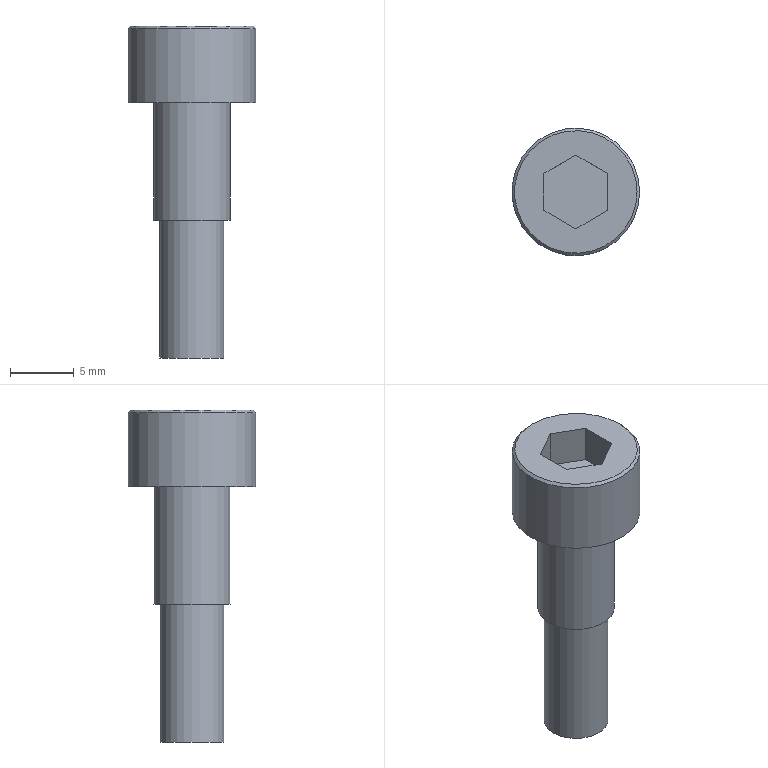Part | STEP file | M3-10_id562_x_t | 1 solid | 15 faces | box 10 x 10 x 26 mm | volume 877.848 mm3 | plane 11 | cylinder 3 | cone 1 | commonest cylinder face diameters 5 x1 6 x1 10 x1
STEP:
#1=CARTESIAN_POINT('',(-317.5,-147.5,-54.182));
#2=VERTEX_POINT('',#1);
#3=CARTESIAN_POINT('',(-315.,-147.5,-54.182));
#4=DIRECTION('',(0.,0.,-1.));
#5=DIRECTION('',(-1.,0.,0.));
#6=AXIS2_PLACEMENT_3D('',#3,#4,#5);
#7=CIRCLE('',#6,2.5);
#8=EDGE_CURVE('',#2,#2,#7,.T.);
#9=ORIENTED_EDGE('',*,*,#8,.F.);
#10=EDGE_LOOP('',(#9));
#11=FACE_BOUND('',#10,.T.);
#12=CARTESIAN_POINT('',(-312.,-147.5,-54.182));
#13=VERTEX_POINT('',#12);
#14=CARTESIAN_POINT('',(-315.,-147.5,-54.182));
#15=DIRECTION('',(0.,0.,1.));
#16=DIRECTION('',(1.,0.,0.));
#17=AXIS2_PLACEMENT_3D('',#14,#15,#16);
#18=CIRCLE('',#17,3.);
#19=EDGE_CURVE('',#13,#13,#18,.T.);
#20=ORIENTED_EDGE('',*,*,#19,.F.);
#21=EDGE_LOOP('',(#20));
#22=FACE_BOUND('',#21,.T.);
#23=CARTESIAN_POINT('',(-315.,-147.5,-54.182));
#24=DIRECTION('',(0.,0.,-1.));
#25=DIRECTION('',(-1.,0.,0.));
#26=AXIS2_PLACEMENT_3D('',#23,#24,#25);
#27=PLANE('',#26);
#28=ADVANCED_FACE('',(#11,#22),#27,.T.);
#29=CARTESIAN_POINT('',(-318.,-147.5,-44.982));
#30=VERTEX_POINT('',#29);
#31=CARTESIAN_POINT('',(-315.,-147.5,-44.982));
#32=DIRECTION('',(0.,0.,1.));
#33=DIRECTION('',(-1.,0.,0.));
#34=AXIS2_PLACEMENT_3D('',#31,#32,#33);
#35=CIRCLE('',#34,3.);
#36=EDGE_CURVE('',#30,#30,#35,.T.);
#37=ORIENTED_EDGE('',*,*,#36,.F.);
#38=EDGE_LOOP('',(#37));
#39=FACE_BOUND('',#38,.T.);
#40=ORIENTED_EDGE('',*,*,#19,.T.);
#41=EDGE_LOOP('',(#40));
#42=FACE_BOUND('',#41,.T.);
#43=CARTESIAN_POINT('',(-315.,-147.5,-54.182));
#44=DIRECTION('',(0.,0.,1.));
#45=DIRECTION('',(1.,0.,0.));
#46=AXIS2_PLACEMENT_3D('',#43,#44,#45);
#47=CYLINDRICAL_SURFACE('',#46,3.);
#48=ADVANCED_FACE('',(#39,#42),#47,.T.);
#49=CARTESIAN_POINT('',(-312.5,-147.5,-64.982));
#50=VERTEX_POINT('',#49);
#51=CARTESIAN_POINT('',(-315.,-147.5,-64.982));
#52=DIRECTION('',(0.,0.,1.));
#53=DIRECTION('',(1.,0.,0.));
#54=AXIS2_PLACEMENT_3D('',#51,#52,#53);
#55=CIRCLE('',#54,2.5);
#56=EDGE_CURVE('',#50,#50,#55,.T.);
#57=ORIENTED_EDGE('',*,*,#56,.F.);
#58=EDGE_LOOP('',(#57));
#59=FACE_OUTER_BOUND('',#58,.T.);
#60=CARTESIAN_POINT('',(-315.,-147.5,-64.982));
#61=DIRECTION('',(0.,0.,-1.));
#62=DIRECTION('',(-1.,0.,0.));
#63=AXIS2_PLACEMENT_3D('',#60,#61,#62);
#64=PLANE('',#63);
#65=ADVANCED_FACE('',(#59),#64,.T.);
#66=ORIENTED_EDGE('',*,*,#56,.T.);
#67=EDGE_LOOP('',(#66));
#68=FACE_BOUND('',#67,.T.);
#69=ORIENTED_EDGE('',*,*,#8,.T.);
#70=EDGE_LOOP('',(#69));
#71=FACE_BOUND('',#70,.T.);
#72=CARTESIAN_POINT('',(-315.,-147.5,-54.182));
#73=DIRECTION('',(0.,0.,-1.));
#74=DIRECTION('',(1.,0.,0.));
#75=AXIS2_PLACEMENT_3D('',#72,#73,#74);
#76=CYLINDRICAL_SURFACE('',#75,2.5);
#77=ADVANCED_FACE('',(#68,#71),#76,.T.);
#78=CARTESIAN_POINT('',(-317.5,-146.057,-38.982));
#79=VERTEX_POINT('',#78);
#80=CARTESIAN_POINT('',(-317.5,-148.943,-38.982));
#81=VERTEX_POINT('',#80);
#82=CARTESIAN_POINT('',(-317.5,-146.057,-38.982));
#83=DIRECTION('',(0.,-1.,0.));
#84=VECTOR('',#83,1.);
#85=LINE('',#82,#84);
#86=EDGE_CURVE('',#79,#81,#85,.T.);
#87=ORIENTED_EDGE('',*,*,#86,.F.);
#88=CARTESIAN_POINT('',(-315.,-144.613,-38.982));
#89=VERTEX_POINT('',#88);
#90=CARTESIAN_POINT('',(-315.,-144.613,-38.982));
#91=DIRECTION('',(-0.866,-0.5,0.));
#92=VECTOR('',#91,1.);
#93=LINE('',#90,#92);
#94=EDGE_CURVE('',#89,#79,#93,.T.);
#95=ORIENTED_EDGE('',*,*,#94,.F.);
#96=CARTESIAN_POINT('',(-312.5,-146.057,-38.982));
#97=VERTEX_POINT('',#96);
#98=CARTESIAN_POINT('',(-312.5,-146.057,-38.982));
#99=DIRECTION('',(-0.866,0.5,0.));
#100=VECTOR('',#99,1.);
#101=LINE('',#98,#100);
#102=EDGE_CURVE('',#97,#89,#101,.T.);
#103=ORIENTED_EDGE('',*,*,#102,.F.);
#104=CARTESIAN_POINT('',(-312.5,-148.943,-38.982));
#105=VERTEX_POINT('',#104);
#106=CARTESIAN_POINT('',(-312.5,-148.943,-38.982));
#107=DIRECTION('',(0.,1.,0.));
#108=VECTOR('',#107,1.);
#109=LINE('',#106,#108);
#110=EDGE_CURVE('',#105,#97,#109,.T.);
#111=ORIENTED_EDGE('',*,*,#110,.F.);
#112=CARTESIAN_POINT('',(-315.,-150.387,-38.982));
#113=VERTEX_POINT('',#112);
#114=CARTESIAN_POINT('',(-315.,-150.387,-38.982));
#115=DIRECTION('',(0.866,0.5,0.));
#116=VECTOR('',#115,1.);
#117=LINE('',#114,#116);
#118=EDGE_CURVE('',#113,#105,#117,.T.);
#119=ORIENTED_EDGE('',*,*,#118,.F.);
#120=CARTESIAN_POINT('',(-317.5,-148.943,-38.982));
#121=DIRECTION('',(0.866,-0.5,0.));
#122=VECTOR('',#121,1.);
#123=LINE('',#120,#122);
#124=EDGE_CURVE('',#81,#113,#123,.T.);
#125=ORIENTED_EDGE('',*,*,#124,.F.);
#126=EDGE_LOOP('',(#87,#95,#103,#111,#119,#125));
#127=FACE_BOUND('',#126,.T.);
#128=CARTESIAN_POINT('',(-310.2,-147.5,-38.982));
#129=VERTEX_POINT('',#128);
#130=CARTESIAN_POINT('',(-315.,-147.5,-38.982));
#131=DIRECTION('',(0.,0.,1.));
#132=DIRECTION('',(1.,0.,0.));
#133=AXIS2_PLACEMENT_3D('',#130,#131,#132);
#134=CIRCLE('',#133,4.8);
#135=EDGE_CURVE('',#129,#129,#134,.T.);
#136=ORIENTED_EDGE('',*,*,#135,.T.);
#137=EDGE_LOOP('',(#136));
#138=FACE_BOUND('',#137,.T.);
#139=CARTESIAN_POINT('',(-315.,-147.5,-38.982));
#140=DIRECTION('',(0.,0.,1.));
#141=DIRECTION('',(1.,0.,0.));
#142=AXIS2_PLACEMENT_3D('',#139,#140,#141);
#143=PLANE('',#142);
#144=ADVANCED_FACE('',(#127,#138),#143,.T.);
#145=ORIENTED_EDGE('',*,*,#36,.T.);
#146=EDGE_LOOP('',(#145));
#147=FACE_BOUND('',#146,.T.);
#148=CARTESIAN_POINT('',(-310.,-147.5,-44.982));
#149=VERTEX_POINT('',#148);
#150=CARTESIAN_POINT('',(-315.,-147.5,-44.982));
#151=DIRECTION('',(0.,0.,1.));
#152=DIRECTION('',(1.,0.,0.));
#153=AXIS2_PLACEMENT_3D('',#150,#151,#152);
#154=CIRCLE('',#153,5.);
#155=EDGE_CURVE('',#149,#149,#154,.T.);
#156=ORIENTED_EDGE('',*,*,#155,.F.);
#157=EDGE_LOOP('',(#156));
#158=FACE_BOUND('',#157,.T.);
#159=CARTESIAN_POINT('',(-315.,-147.5,-44.982));
#160=DIRECTION('',(0.,0.,-1.));
#161=DIRECTION('',(-1.,0.,0.));
#162=AXIS2_PLACEMENT_3D('',#159,#160,#161);
#163=PLANE('',#162);
#164=ADVANCED_FACE('',(#147,#158),#163,.T.);
#165=CARTESIAN_POINT('',(-310.,-147.5,-39.182));
#166=VERTEX_POINT('',#165);
#167=CARTESIAN_POINT('',(-315.,-147.5,-39.182));
#168=DIRECTION('',(0.,0.,-1.));
#169=DIRECTION('',(1.,0.,0.));
#170=AXIS2_PLACEMENT_3D('',#167,#168,#169);
#171=CIRCLE('',#170,5.);
#172=EDGE_CURVE('',#166,#166,#171,.T.);
#173=ORIENTED_EDGE('',*,*,#172,.T.);
#174=EDGE_LOOP('',(#173));
#175=FACE_BOUND('',#174,.T.);
#176=ORIENTED_EDGE('',*,*,#155,.T.);
#177=EDGE_LOOP('',(#176));
#178=FACE_BOUND('',#177,.T.);
#179=CARTESIAN_POINT('',(-315.,-147.5,-44.982));
#180=DIRECTION('',(0.,0.,1.));
#181=DIRECTION('',(1.,0.,0.));
#182=AXIS2_PLACEMENT_3D('',#179,#180,#181);
#183=CYLINDRICAL_SURFACE('',#182,5.);
#184=ADVANCED_FACE('',(#175,#178),#183,.T.);
#185=ORIENTED_EDGE('',*,*,#135,.F.);
#186=EDGE_LOOP('',(#185));
#187=FACE_BOUND('',#186,.T.);
#188=ORIENTED_EDGE('',*,*,#172,.F.);
#189=EDGE_LOOP('',(#188));
#190=FACE_BOUND('',#189,.T.);
#191=CARTESIAN_POINT('',(-315.,-147.5,-39.182));
#192=DIRECTION('',(0.,0.,-1.));
#193=DIRECTION('',(-1.,0.,0.));
#194=AXIS2_PLACEMENT_3D('',#191,#192,#193);
#195=CONICAL_SURFACE('',#194,5.,45.);
#196=ADVANCED_FACE('',(#187,#190),#195,.T.);
#197=ORIENTED_EDGE('',*,*,#86,.T.);
#198=CARTESIAN_POINT('',(-317.5,-148.943,-41.982));
#199=VERTEX_POINT('',#198);
#200=CARTESIAN_POINT('',(-317.5,-148.943,-41.982));
#201=DIRECTION('',(0.,0.,-1.));
#202=VECTOR('',#201,1.);
#203=LINE('',#200,#202);
#204=EDGE_CURVE('',#81,#199,#203,.T.);
#205=ORIENTED_EDGE('',*,*,#204,.T.);
#206=CARTESIAN_POINT('',(-317.5,-146.057,-41.982));
#207=VERTEX_POINT('',#206);
#208=CARTESIAN_POINT('',(-317.5,-146.057,-41.982));
#209=DIRECTION('',(0.,1.,0.));
#210=VECTOR('',#209,1.);
#211=LINE('',#208,#210);
#212=EDGE_CURVE('',#199,#207,#211,.T.);
#213=ORIENTED_EDGE('',*,*,#212,.T.);
#214=CARTESIAN_POINT('',(-317.5,-146.057,-41.982));
#215=DIRECTION('',(0.,0.,-1.));
#216=VECTOR('',#215,1.);
#217=LINE('',#214,#216);
#218=EDGE_CURVE('',#79,#207,#217,.T.);
#219=ORIENTED_EDGE('',*,*,#218,.F.);
#220=EDGE_LOOP('',(#197,#205,#213,#219));
#221=FACE_OUTER_BOUND('',#220,.T.);
#222=CARTESIAN_POINT('',(-317.5,-146.057,-41.982));
#223=DIRECTION('',(-1.,0.,0.));
#224=DIRECTION('',(0.,-1.,0.));
#225=AXIS2_PLACEMENT_3D('',#222,#223,#224);
#226=PLANE('',#225);
#227=ADVANCED_FACE('',(#221),#226,.F.);
#228=ORIENTED_EDGE('',*,*,#124,.T.);
#229=CARTESIAN_POINT('',(-315.,-150.387,-41.982));
#230=VERTEX_POINT('',#229);
#231=CARTESIAN_POINT('',(-315.,-150.387,-41.982));
#232=DIRECTION('',(0.,0.,-1.));
#233=VECTOR('',#232,1.);
#234=LINE('',#231,#233);
#235=EDGE_CURVE('',#113,#230,#234,.T.);
#236=ORIENTED_EDGE('',*,*,#235,.T.);
#237=CARTESIAN_POINT('',(-317.5,-148.943,-41.982));
#238=DIRECTION('',(-0.866,0.5,0.));
#239=VECTOR('',#238,1.);
#240=LINE('',#237,#239);
#241=EDGE_CURVE('',#230,#199,#240,.T.);
#242=ORIENTED_EDGE('',*,*,#241,.T.);
#243=ORIENTED_EDGE('',*,*,#204,.F.);
#244=EDGE_LOOP('',(#228,#236,#242,#243));
#245=FACE_OUTER_BOUND('',#244,.T.);
#246=CARTESIAN_POINT('',(-317.5,-148.943,-41.982));
#247=DIRECTION('',(-0.5,-0.866,0.));
#248=DIRECTION('',(0.866,-0.5,0.));
#249=AXIS2_PLACEMENT_3D('',#246,#247,#248);
#250=PLANE('',#249);
#251=ADVANCED_FACE('',(#245),#250,.F.);
#252=ORIENTED_EDGE('',*,*,#118,.T.);
#253=CARTESIAN_POINT('',(-312.5,-148.943,-41.982));
#254=VERTEX_POINT('',#253);
#255=CARTESIAN_POINT('',(-312.5,-148.943,-41.982));
#256=DIRECTION('',(0.,0.,-1.));
#257=VECTOR('',#256,1.);
#258=LINE('',#255,#257);
#259=EDGE_CURVE('',#105,#254,#258,.T.);
#260=ORIENTED_EDGE('',*,*,#259,.T.);
#261=CARTESIAN_POINT('',(-315.,-150.387,-41.982));
#262=DIRECTION('',(-0.866,-0.5,0.));
#263=VECTOR('',#262,1.);
#264=LINE('',#261,#263);
#265=EDGE_CURVE('',#254,#230,#264,.T.);
#266=ORIENTED_EDGE('',*,*,#265,.T.);
#267=ORIENTED_EDGE('',*,*,#235,.F.);
#268=EDGE_LOOP('',(#252,#260,#266,#267));
#269=FACE_OUTER_BOUND('',#268,.T.);
#270=CARTESIAN_POINT('',(-315.,-150.387,-41.982));
#271=DIRECTION('',(0.5,-0.866,0.));
#272=DIRECTION('',(0.866,0.5,0.));
#273=AXIS2_PLACEMENT_3D('',#270,#271,#272);
#274=PLANE('',#273);
#275=ADVANCED_FACE('',(#269),#274,.F.);
#276=ORIENTED_EDGE('',*,*,#110,.T.);
#277=CARTESIAN_POINT('',(-312.5,-146.057,-41.982));
#278=VERTEX_POINT('',#277);
#279=CARTESIAN_POINT('',(-312.5,-146.057,-41.982));
#280=DIRECTION('',(0.,0.,-1.));
#281=VECTOR('',#280,1.);
#282=LINE('',#279,#281);
#283=EDGE_CURVE('',#97,#278,#282,.T.);
#284=ORIENTED_EDGE('',*,*,#283,.T.);
#285=CARTESIAN_POINT('',(-312.5,-148.943,-41.982));
#286=DIRECTION('',(0.,-1.,0.));
#287=VECTOR('',#286,1.);
#288=LINE('',#285,#287);
#289=EDGE_CURVE('',#278,#254,#288,.T.);
#290=ORIENTED_EDGE('',*,*,#289,.T.);
#291=ORIENTED_EDGE('',*,*,#259,.F.);
#292=EDGE_LOOP('',(#276,#284,#290,#291));
#293=FACE_OUTER_BOUND('',#292,.T.);
#294=CARTESIAN_POINT('',(-312.5,-148.943,-41.982));
#295=DIRECTION('',(1.,0.,0.));
#296=DIRECTION('',(0.,1.,0.));
#297=AXIS2_PLACEMENT_3D('',#294,#295,#296);
#298=PLANE('',#297);
#299=ADVANCED_FACE('',(#293),#298,.F.);
#300=ORIENTED_EDGE('',*,*,#102,.T.);
#301=CARTESIAN_POINT('',(-315.,-144.613,-41.982));
#302=VERTEX_POINT('',#301);
#303=CARTESIAN_POINT('',(-315.,-144.613,-41.982));
#304=DIRECTION('',(0.,0.,-1.));
#305=VECTOR('',#304,1.);
#306=LINE('',#303,#305);
#307=EDGE_CURVE('',#89,#302,#306,.T.);
#308=ORIENTED_EDGE('',*,*,#307,.T.);
#309=CARTESIAN_POINT('',(-312.5,-146.057,-41.982));
#310=DIRECTION('',(0.866,-0.5,0.));
#311=VECTOR('',#310,1.);
#312=LINE('',#309,#311);
#313=EDGE_CURVE('',#302,#278,#312,.T.);
#314=ORIENTED_EDGE('',*,*,#313,.T.);
#315=ORIENTED_EDGE('',*,*,#283,.F.);
#316=EDGE_LOOP('',(#300,#308,#314,#315));
#317=FACE_OUTER_BOUND('',#316,.T.);
#318=CARTESIAN_POINT('',(-312.5,-146.057,-41.982));
#319=DIRECTION('',(0.5,0.866,0.));
#320=DIRECTION('',(-0.866,0.5,0.));
#321=AXIS2_PLACEMENT_3D('',#318,#319,#320);
#322=PLANE('',#321);
#323=ADVANCED_FACE('',(#317),#322,.F.);
#324=ORIENTED_EDGE('',*,*,#94,.T.);
#325=ORIENTED_EDGE('',*,*,#218,.T.);
#326=CARTESIAN_POINT('',(-315.,-144.613,-41.982));
#327=DIRECTION('',(0.866,0.5,0.));
#328=VECTOR('',#327,1.);
#329=LINE('',#326,#328);
#330=EDGE_CURVE('',#207,#302,#329,.T.);
#331=ORIENTED_EDGE('',*,*,#330,.T.);
#332=ORIENTED_EDGE('',*,*,#307,.F.);
#333=EDGE_LOOP('',(#324,#325,#331,#332));
#334=FACE_OUTER_BOUND('',#333,.T.);
#335=CARTESIAN_POINT('',(-315.,-144.613,-41.982));
#336=DIRECTION('',(-0.5,0.866,0.));
#337=DIRECTION('',(-0.866,-0.5,0.));
#338=AXIS2_PLACEMENT_3D('',#335,#336,#337);
#339=PLANE('',#338);
#340=ADVANCED_FACE('',(#334),#339,.F.);
#341=ORIENTED_EDGE('',*,*,#212,.F.);
#342=ORIENTED_EDGE('',*,*,#241,.F.);
#343=ORIENTED_EDGE('',*,*,#265,.F.);
#344=ORIENTED_EDGE('',*,*,#289,.F.);
#345=ORIENTED_EDGE('',*,*,#313,.F.);
#346=ORIENTED_EDGE('',*,*,#330,.F.);
#347=EDGE_LOOP('',(#341,#342,#343,#344,#345,#346));
#348=FACE_OUTER_BOUND('',#347,.T.);
#349=CARTESIAN_POINT('',(-315.,-147.5,-41.982));
#350=DIRECTION('',(0.,0.,1.));
#351=DIRECTION('',(1.,0.,0.));
#352=AXIS2_PLACEMENT_3D('',#349,#350,#351);
#353=PLANE('',#352);
#354=ADVANCED_FACE('',(#348),#353,.T.);
#355=CLOSED_SHELL('',(#28,#48,#65,#77,#144,#164,#184,#196,#227,#251,#275,#299,#323,#340,#354));
#356=MANIFOLD_SOLID_BREP('',#355);
#357=(LENGTH_UNIT()NAMED_UNIT(*)SI_UNIT(.MILLI.,.METRE.));
#358=UNCERTAINTY_MEASURE_WITH_UNIT(LENGTH_MEASURE(0.00002),#357,'','');
#359=(NAMED_UNIT(*)PLANE_ANGLE_UNIT()SI_UNIT($,.RADIAN.));
#360=PLANE_ANGLE_MEASURE_WITH_UNIT(PLANE_ANGLE_MEASURE(0.01745),#359);
#361=DIMENSIONAL_EXPONENTS(0.,0.,0.,0.,0.,0.,0.);
#362=(CONVERSION_BASED_UNIT('DEGREE',#360)NAMED_UNIT(#361)PLANE_ANGLE_UNIT());
#363=(NAMED_UNIT(*)SI_UNIT($,.STERADIAN.)SOLID_ANGLE_UNIT());
#364=(GEOMETRIC_REPRESENTATION_CONTEXT(3)GLOBAL_UNCERTAINTY_ASSIGNED_CONTEXT((#358))GLOBAL_UNIT_ASSIGNED_CONTEXT((#357,#362,#363))REPRESENTATION_CONTEXT('',''));
#365=ADVANCED_BREP_SHAPE_REPRESENTATION('',(#356),#364);